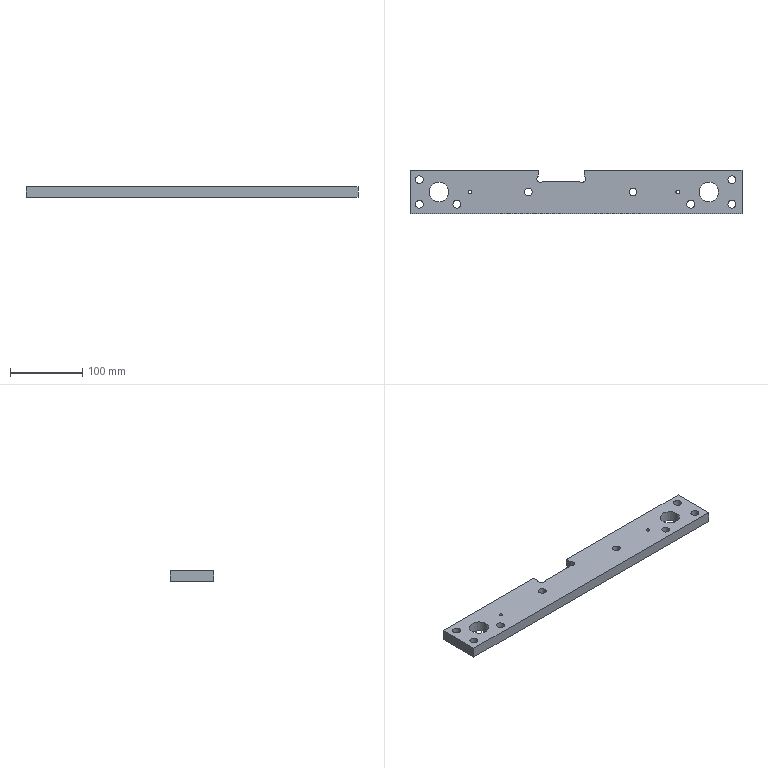Part | NX | features LIN_SOLID_COLOR 2 | 1 solid | 24 faces | box 460 x 60 x 15 mm | volume 369804 mm3 | cylinder 14 | plane 10 | commonest cylinder face diameters 11 x8 5.2 x2 10 x2 27 x2
STEP:
#1=CARTESIAN_POINT('',(813.,-110.,-46.5));
#2=VERTEX_POINT('',#1);
#3=CARTESIAN_POINT('',(594.5,-110.,-46.5));
#4=VERTEX_POINT('',#3);
#5=CARTESIAN_POINT('',(667.,-110.,-46.5));
#6=DIRECTION('',(-1.,0.,0.));
#7=VECTOR('',#6,1000.);
#8=LINE('',#5,#7);
#9=EDGE_CURVE('',#2,#4,#8,.T.);
#10=ORIENTED_EDGE('',*,*,#9,.T.);
#11=CARTESIAN_POINT('',(594.5,-110.,-31.5));
#12=VERTEX_POINT('',#11);
#13=CARTESIAN_POINT('',(594.5,-110.,-91.5));
#14=DIRECTION('',(0.,0.,1.));
#15=VECTOR('',#14,1000.);
#16=LINE('',#13,#15);
#17=EDGE_CURVE('',#12,#4,#16,.F.);
#18=ORIENTED_EDGE('',*,*,#17,.F.);
#19=CARTESIAN_POINT('',(813.,-110.,-31.5));
#20=VERTEX_POINT('',#19);
#21=CARTESIAN_POINT('',(667.,-110.,-31.5));
#22=DIRECTION('',(-1.,0.,0.));
#23=VECTOR('',#22,1000.);
#24=LINE('',#21,#23);
#25=EDGE_CURVE('',#12,#20,#24,.F.);
#26=ORIENTED_EDGE('',*,*,#25,.T.);
#27=CARTESIAN_POINT('',(813.,-110.,12.5));
#28=DIRECTION('',(0.,0.,1.));
#29=VECTOR('',#28,1000.);
#30=LINE('',#27,#29);
#31=EDGE_CURVE('',#2,#20,#30,.T.);
#32=ORIENTED_EDGE('',*,*,#31,.F.);
#33=EDGE_LOOP('',(#10,#18,#26,#32));
#34=FACE_BOUND('',#33,.T.);
#35=CARTESIAN_POINT('',(667.,-110.,-56.5));
#36=DIRECTION('',(0.,1.,0.));
#37=DIRECTION('',(0.,0.,1.));
#38=AXIS2_PLACEMENT_3D('',#35,#36,#37);
#39=PLANE('',#38);
#40=ADVANCED_FACE('',(#34),#39,.T.);
#41=CARTESIAN_POINT('',(353.,-110.,-31.5));
#42=VERTEX_POINT('',#41);
#43=CARTESIAN_POINT('',(530.5,-110.,-31.5));
#44=VERTEX_POINT('',#43);
#45=CARTESIAN_POINT('',(667.,-110.,-31.5));
#46=DIRECTION('',(-1.,0.,0.));
#47=VECTOR('',#46,1000.);
#48=LINE('',#45,#47);
#49=EDGE_CURVE('',#42,#44,#48,.F.);
#50=ORIENTED_EDGE('',*,*,#49,.T.);
#51=CARTESIAN_POINT('',(530.5,-110.,-46.5));
#52=VERTEX_POINT('',#51);
#53=CARTESIAN_POINT('',(530.5,-110.,-91.5));
#54=DIRECTION('',(0.,0.,1.));
#55=VECTOR('',#54,1000.);
#56=LINE('',#53,#55);
#57=EDGE_CURVE('',#52,#44,#56,.T.);
#58=ORIENTED_EDGE('',*,*,#57,.F.);
#59=CARTESIAN_POINT('',(353.,-110.,-46.5));
#60=VERTEX_POINT('',#59);
#61=CARTESIAN_POINT('',(667.,-110.,-46.5));
#62=DIRECTION('',(-1.,0.,0.));
#63=VECTOR('',#62,1000.);
#64=LINE('',#61,#63);
#65=EDGE_CURVE('',#52,#60,#64,.T.);
#66=ORIENTED_EDGE('',*,*,#65,.T.);
#67=CARTESIAN_POINT('',(353.,-110.,-56.5));
#68=DIRECTION('',(0.,0.,1.));
#69=VECTOR('',#68,1000.);
#70=LINE('',#67,#69);
#71=EDGE_CURVE('',#60,#42,#70,.T.);
#72=ORIENTED_EDGE('',*,*,#71,.T.);
#73=EDGE_LOOP('',(#50,#58,#66,#72));
#74=FACE_BOUND('',#73,.T.);
#75=CARTESIAN_POINT('',(667.,-110.,-56.5));
#76=DIRECTION('',(0.,1.,0.));
#77=DIRECTION('',(0.,0.,1.));
#78=AXIS2_PLACEMENT_3D('',#75,#76,#77);
#79=PLANE('',#78);
#80=ADVANCED_FACE('',(#74),#79,.T.);
#81=CARTESIAN_POINT('',(406.5,-140.,-31.5));
#82=VERTEX_POINT('',#81);
#83=CARTESIAN_POINT('',(393.,-140.,-31.5));
#84=DIRECTION('',(0.,0.,1.));
#85=DIRECTION('',(1.,0.,0.));
#86=AXIS2_PLACEMENT_3D('',#83,#84,#85);
#87=CIRCLE('',#86,13.5);
#88=EDGE_CURVE('',#82,#82,#87,.F.);
#89=ORIENTED_EDGE('',*,*,#88,.T.);
#90=EDGE_LOOP('',(#89));
#91=FACE_BOUND('',#90,.T.);
#92=CARTESIAN_POINT('',(753.5,-140.,-31.5));
#93=VERTEX_POINT('',#92);
#94=CARTESIAN_POINT('',(767.,-140.,-31.5));
#95=DIRECTION('',(0.,0.,-1.));
#96=DIRECTION('',(-1.,0.,0.));
#97=AXIS2_PLACEMENT_3D('',#94,#95,#96);
#98=CIRCLE('',#97,13.5);
#99=EDGE_CURVE('',#93,#93,#98,.F.);
#100=ORIENTED_EDGE('',*,*,#99,.F.);
#101=EDGE_LOOP('',(#100));
#102=FACE_BOUND('',#101,.T.);
#103=CARTESIAN_POINT('',(371.5,-123.,-31.5));
#104=VERTEX_POINT('',#103);
#105=CARTESIAN_POINT('',(366.,-123.,-31.5));
#106=DIRECTION('',(0.,0.,1.));
#107=DIRECTION('',(1.,0.,0.));
#108=AXIS2_PLACEMENT_3D('',#105,#106,#107);
#109=CIRCLE('',#108,5.5);
#110=EDGE_CURVE('',#104,#104,#109,.T.);
#111=ORIENTED_EDGE('',*,*,#110,.F.);
#112=EDGE_LOOP('',(#111));
#113=FACE_BOUND('',#112,.T.);
#114=CARTESIAN_POINT('',(522.5,-140.,-31.5));
#115=VERTEX_POINT('',#114);
#116=CARTESIAN_POINT('',(517.,-140.,-31.5));
#117=DIRECTION('',(0.,0.,1.));
#118=DIRECTION('',(1.,0.,0.));
#119=AXIS2_PLACEMENT_3D('',#116,#117,#118);
#120=CIRCLE('',#119,5.5);
#121=EDGE_CURVE('',#115,#115,#120,.T.);
#122=ORIENTED_EDGE('',*,*,#121,.F.);
#123=EDGE_LOOP('',(#122));
#124=FACE_BOUND('',#123,.T.);
#125=CARTESIAN_POINT('',(747.497,-157.,-31.5));
#126=VERTEX_POINT('',#125);
#127=CARTESIAN_POINT('',(741.997,-157.,-31.5));
#128=DIRECTION('',(0.,0.,1.));
#129=DIRECTION('',(1.,0.,0.));
#130=AXIS2_PLACEMENT_3D('',#127,#128,#129);
#131=CIRCLE('',#130,5.5);
#132=EDGE_CURVE('',#126,#126,#131,.T.);
#133=ORIENTED_EDGE('',*,*,#132,.F.);
#134=EDGE_LOOP('',(#133));
#135=FACE_BOUND('',#134,.T.);
#136=CARTESIAN_POINT('',(804.5,-157.,-31.5));
#137=VERTEX_POINT('',#136);
#138=CARTESIAN_POINT('',(799.,-157.,-31.5));
#139=DIRECTION('',(0.,0.,1.));
#140=DIRECTION('',(1.,0.,0.));
#141=AXIS2_PLACEMENT_3D('',#138,#139,#140);
#142=CIRCLE('',#141,5.5);
#143=EDGE_CURVE('',#137,#137,#142,.T.);
#144=ORIENTED_EDGE('',*,*,#143,.F.);
#145=EDGE_LOOP('',(#144));
#146=FACE_BOUND('',#145,.T.);
#147=CARTESIAN_POINT('',(804.5,-123.,-31.5));
#148=VERTEX_POINT('',#147);
#149=CARTESIAN_POINT('',(799.,-123.,-31.5));
#150=DIRECTION('',(0.,0.,1.));
#151=DIRECTION('',(1.,0.,0.));
#152=AXIS2_PLACEMENT_3D('',#149,#150,#151);
#153=CIRCLE('',#152,5.5);
#154=EDGE_CURVE('',#148,#148,#153,.T.);
#155=ORIENTED_EDGE('',*,*,#154,.F.);
#156=EDGE_LOOP('',(#155));
#157=FACE_BOUND('',#156,.T.);
#158=CARTESIAN_POINT('',(371.5,-157.,-31.5));
#159=VERTEX_POINT('',#158);
#160=CARTESIAN_POINT('',(366.,-157.,-31.5));
#161=DIRECTION('',(0.,0.,1.));
#162=DIRECTION('',(1.,0.,0.));
#163=AXIS2_PLACEMENT_3D('',#160,#161,#162);
#164=CIRCLE('',#163,5.5);
#165=EDGE_CURVE('',#159,#159,#164,.T.);
#166=ORIENTED_EDGE('',*,*,#165,.F.);
#167=EDGE_LOOP('',(#166));
#168=FACE_BOUND('',#167,.T.);
#169=CARTESIAN_POINT('',(423.503,-157.,-31.5));
#170=VERTEX_POINT('',#169);
#171=CARTESIAN_POINT('',(418.003,-157.,-31.5));
#172=DIRECTION('',(0.,0.,1.));
#173=DIRECTION('',(1.,0.,0.));
#174=AXIS2_PLACEMENT_3D('',#171,#172,#173);
#175=CIRCLE('',#174,5.5);
#176=EDGE_CURVE('',#170,#170,#175,.T.);
#177=ORIENTED_EDGE('',*,*,#176,.F.);
#178=EDGE_LOOP('',(#177));
#179=FACE_BOUND('',#178,.T.);
#180=CARTESIAN_POINT('',(726.6,-140.,-31.5));
#181=VERTEX_POINT('',#180);
#182=CARTESIAN_POINT('',(724.,-140.,-31.5));
#183=DIRECTION('',(0.,0.,1.));
#184=DIRECTION('',(1.,0.,0.));
#185=AXIS2_PLACEMENT_3D('',#182,#183,#184);
#186=CIRCLE('',#185,2.6);
#187=EDGE_CURVE('',#181,#181,#186,.T.);
#188=ORIENTED_EDGE('',*,*,#187,.F.);
#189=EDGE_LOOP('',(#188));
#190=FACE_BOUND('',#189,.T.);
#191=CARTESIAN_POINT('',(438.6,-140.,-31.5));
#192=VERTEX_POINT('',#191);
#193=CARTESIAN_POINT('',(436.,-140.,-31.5));
#194=DIRECTION('',(0.,0.,1.));
#195=DIRECTION('',(1.,0.,0.));
#196=AXIS2_PLACEMENT_3D('',#193,#194,#195);
#197=CIRCLE('',#196,2.6);
#198=EDGE_CURVE('',#192,#192,#197,.T.);
#199=ORIENTED_EDGE('',*,*,#198,.F.);
#200=EDGE_LOOP('',(#199));
#201=FACE_BOUND('',#200,.T.);
#202=CARTESIAN_POINT('',(667.5,-140.,-31.5));
#203=VERTEX_POINT('',#202);
#204=CARTESIAN_POINT('',(662.,-140.,-31.5));
#205=DIRECTION('',(0.,0.,1.));
#206=DIRECTION('',(1.,0.,0.));
#207=AXIS2_PLACEMENT_3D('',#204,#205,#206);
#208=CIRCLE('',#207,5.5);
#209=EDGE_CURVE('',#203,#203,#208,.T.);
#210=ORIENTED_EDGE('',*,*,#209,.F.);
#211=EDGE_LOOP('',(#210));
#212=FACE_BOUND('',#211,.T.);
#213=ORIENTED_EDGE('',*,*,#25,.F.);
#214=CARTESIAN_POINT('',(594.5,-117.961,-31.5));
#215=VERTEX_POINT('',#214);
#216=CARTESIAN_POINT('',(594.5,-140.,-31.5));
#217=DIRECTION('',(0.,-1.,0.));
#218=VECTOR('',#217,1000.);
#219=LINE('',#216,#218);
#220=EDGE_CURVE('',#215,#12,#219,.F.);
#221=ORIENTED_EDGE('',*,*,#220,.F.);
#222=CARTESIAN_POINT('',(587.461,-125.,-31.5));
#223=VERTEX_POINT('',#222);
#224=CARTESIAN_POINT('',(591.318,-121.818,-31.5));
#225=DIRECTION('',(0.,0.,1.));
#226=DIRECTION('',(1.,0.,0.));
#227=AXIS2_PLACEMENT_3D('',#224,#225,#226);
#228=CIRCLE('',#227,5.);
#229=EDGE_CURVE('',#223,#215,#228,.T.);
#230=ORIENTED_EDGE('',*,*,#229,.F.);
#231=CARTESIAN_POINT('',(537.539,-125.,-31.5));
#232=VERTEX_POINT('',#231);
#233=CARTESIAN_POINT('',(667.,-125.,-31.5));
#234=DIRECTION('',(-1.,0.,0.));
#235=VECTOR('',#234,1000.);
#236=LINE('',#233,#235);
#237=EDGE_CURVE('',#232,#223,#236,.F.);
#238=ORIENTED_EDGE('',*,*,#237,.F.);
#239=CARTESIAN_POINT('',(530.5,-117.961,-31.5));
#240=VERTEX_POINT('',#239);
#241=CARTESIAN_POINT('',(533.682,-121.818,-31.5));
#242=DIRECTION('',(0.,0.,1.));
#243=DIRECTION('',(1.,0.,0.));
#244=AXIS2_PLACEMENT_3D('',#241,#242,#243);
#245=CIRCLE('',#244,5.);
#246=EDGE_CURVE('',#232,#240,#245,.F.);
#247=ORIENTED_EDGE('',*,*,#246,.T.);
#248=CARTESIAN_POINT('',(530.5,-140.,-31.5));
#249=DIRECTION('',(0.,1.,0.));
#250=VECTOR('',#249,1000.);
#251=LINE('',#248,#250);
#252=EDGE_CURVE('',#240,#44,#251,.T.);
#253=ORIENTED_EDGE('',*,*,#252,.T.);
#254=ORIENTED_EDGE('',*,*,#49,.F.);
#255=CARTESIAN_POINT('',(353.,-170.,-31.5));
#256=VERTEX_POINT('',#255);
#257=CARTESIAN_POINT('',(353.,-30.,-31.5));
#258=DIRECTION('',(0.,1.,0.));
#259=VECTOR('',#258,1000.);
#260=LINE('',#257,#259);
#261=EDGE_CURVE('',#256,#42,#260,.T.);
#262=ORIENTED_EDGE('',*,*,#261,.F.);
#263=CARTESIAN_POINT('',(813.,-170.,-31.5));
#264=VERTEX_POINT('',#263);
#265=CARTESIAN_POINT('',(667.,-170.,-31.5));
#266=DIRECTION('',(1.,0.,0.));
#267=VECTOR('',#266,1000.);
#268=LINE('',#265,#267);
#269=EDGE_CURVE('',#264,#256,#268,.F.);
#270=ORIENTED_EDGE('',*,*,#269,.F.);
#271=CARTESIAN_POINT('',(813.,-140.,-31.5));
#272=DIRECTION('',(0.,1.,0.));
#273=VECTOR('',#272,1000.);
#274=LINE('',#271,#273);
#275=EDGE_CURVE('',#264,#20,#274,.T.);
#276=ORIENTED_EDGE('',*,*,#275,.T.);
#277=EDGE_LOOP('',(#213,#221,#230,#238,#247,#253,#254,#262,#270,#276));
#278=FACE_BOUND('',#277,.T.);
#279=CARTESIAN_POINT('',(667.,-140.,-31.5));
#280=DIRECTION('',(0.,0.,1.));
#281=DIRECTION('',(-1.,0.,0.));
#282=AXIS2_PLACEMENT_3D('',#279,#280,#281);
#283=PLANE('',#282);
#284=ADVANCED_FACE('',(#91,#102,#113,#124,#135,#146,#157,#168,#179,#190,#201,#212,#278),#283,.T.);
#285=CARTESIAN_POINT('',(433.4,-140.,-46.5));
#286=VERTEX_POINT('',#285);
#287=CARTESIAN_POINT('',(436.,-140.,-46.5));
#288=DIRECTION('',(0.,0.,-1.));
#289=DIRECTION('',(-1.,0.,0.));
#290=AXIS2_PLACEMENT_3D('',#287,#288,#289);
#291=CIRCLE('',#290,2.6);
#292=EDGE_CURVE('',#286,#286,#291,.F.);
#293=ORIENTED_EDGE('',*,*,#292,.T.);
#294=EDGE_LOOP('',(#293));
#295=FACE_BOUND('',#294,.T.);
#296=CARTESIAN_POINT('',(379.5,-140.,-46.5));
#297=VERTEX_POINT('',#296);
#298=CARTESIAN_POINT('',(393.,-140.,-46.5));
#299=DIRECTION('',(0.,0.,-1.));
#300=DIRECTION('',(-1.,0.,0.));
#301=AXIS2_PLACEMENT_3D('',#298,#299,#300);
#302=CIRCLE('',#301,13.5);
#303=EDGE_CURVE('',#297,#297,#302,.F.);
#304=ORIENTED_EDGE('',*,*,#303,.T.);
#305=EDGE_LOOP('',(#304));
#306=FACE_BOUND('',#305,.T.);
#307=CARTESIAN_POINT('',(753.5,-140.,-46.5));
#308=VERTEX_POINT('',#307);
#309=CARTESIAN_POINT('',(767.,-140.,-46.5));
#310=DIRECTION('',(0.,0.,-1.));
#311=DIRECTION('',(-1.,0.,0.));
#312=AXIS2_PLACEMENT_3D('',#309,#310,#311);
#313=CIRCLE('',#312,13.5);
#314=EDGE_CURVE('',#308,#308,#313,.T.);
#315=ORIENTED_EDGE('',*,*,#314,.F.);
#316=EDGE_LOOP('',(#315));
#317=FACE_BOUND('',#316,.T.);
#318=CARTESIAN_POINT('',(360.5,-123.,-46.5));
#319=VERTEX_POINT('',#318);
#320=CARTESIAN_POINT('',(366.,-123.,-46.5));
#321=DIRECTION('',(0.,0.,-1.));
#322=DIRECTION('',(-1.,0.,0.));
#323=AXIS2_PLACEMENT_3D('',#320,#321,#322);
#324=CIRCLE('',#323,5.5);
#325=EDGE_CURVE('',#319,#319,#324,.T.);
#326=ORIENTED_EDGE('',*,*,#325,.F.);
#327=EDGE_LOOP('',(#326));
#328=FACE_BOUND('',#327,.T.);
#329=CARTESIAN_POINT('',(511.5,-140.,-46.5));
#330=VERTEX_POINT('',#329);
#331=CARTESIAN_POINT('',(517.,-140.,-46.5));
#332=DIRECTION('',(0.,0.,-1.));
#333=DIRECTION('',(-1.,0.,0.));
#334=AXIS2_PLACEMENT_3D('',#331,#332,#333);
#335=CIRCLE('',#334,5.5);
#336=EDGE_CURVE('',#330,#330,#335,.T.);
#337=ORIENTED_EDGE('',*,*,#336,.F.);
#338=EDGE_LOOP('',(#337));
#339=FACE_BOUND('',#338,.T.);
#340=CARTESIAN_POINT('',(736.497,-157.,-46.5));
#341=VERTEX_POINT('',#340);
#342=CARTESIAN_POINT('',(741.997,-157.,-46.5));
#343=DIRECTION('',(0.,0.,-1.));
#344=DIRECTION('',(-1.,0.,0.));
#345=AXIS2_PLACEMENT_3D('',#342,#343,#344);
#346=CIRCLE('',#345,5.5);
#347=EDGE_CURVE('',#341,#341,#346,.T.);
#348=ORIENTED_EDGE('',*,*,#347,.F.);
#349=EDGE_LOOP('',(#348));
#350=FACE_BOUND('',#349,.T.);
#351=CARTESIAN_POINT('',(793.5,-157.,-46.5));
#352=VERTEX_POINT('',#351);
#353=CARTESIAN_POINT('',(799.,-157.,-46.5));
#354=DIRECTION('',(0.,0.,-1.));
#355=DIRECTION('',(-1.,0.,0.));
#356=AXIS2_PLACEMENT_3D('',#353,#354,#355);
#357=CIRCLE('',#356,5.5);
#358=EDGE_CURVE('',#352,#352,#357,.T.);
#359=ORIENTED_EDGE('',*,*,#358,.F.);
#360=EDGE_LOOP('',(#359));
#361=FACE_BOUND('',#360,.T.);
#362=CARTESIAN_POINT('',(793.5,-123.,-46.5));
#363=VERTEX_POINT('',#362);
#364=CARTESIAN_POINT('',(799.,-123.,-46.5));
#365=DIRECTION('',(0.,0.,-1.));
#366=DIRECTION('',(-1.,0.,0.));
#367=AXIS2_PLACEMENT_3D('',#364,#365,#366);
#368=CIRCLE('',#367,5.5);
#369=EDGE_CURVE('',#363,#363,#368,.T.);
#370=ORIENTED_EDGE('',*,*,#369,.F.);
#371=EDGE_LOOP('',(#370));
#372=FACE_BOUND('',#371,.T.);
#373=CARTESIAN_POINT('',(360.5,-157.,-46.5));
#374=VERTEX_POINT('',#373);
#375=CARTESIAN_POINT('',(366.,-157.,-46.5));
#376=DIRECTION('',(0.,0.,-1.));
#377=DIRECTION('',(-1.,0.,0.));
#378=AXIS2_PLACEMENT_3D('',#375,#376,#377);
#379=CIRCLE('',#378,5.5);
#380=EDGE_CURVE('',#374,#374,#379,.T.);
#381=ORIENTED_EDGE('',*,*,#380,.F.);
#382=EDGE_LOOP('',(#381));
#383=FACE_BOUND('',#382,.T.);
#384=CARTESIAN_POINT('',(412.503,-157.,-46.5));
#385=VERTEX_POINT('',#384);
#386=CARTESIAN_POINT('',(418.003,-157.,-46.5));
#387=DIRECTION('',(0.,0.,-1.));
#388=DIRECTION('',(-1.,0.,0.));
#389=AXIS2_PLACEMENT_3D('',#386,#387,#388);
#390=CIRCLE('',#389,5.5);
#391=EDGE_CURVE('',#385,#385,#390,.T.);
#392=ORIENTED_EDGE('',*,*,#391,.F.);
#393=EDGE_LOOP('',(#392));
#394=FACE_BOUND('',#393,.T.);
#395=CARTESIAN_POINT('',(721.4,-140.,-46.5));
#396=VERTEX_POINT('',#395);
#397=CARTESIAN_POINT('',(724.,-140.,-46.5));
#398=DIRECTION('',(0.,0.,-1.));
#399=DIRECTION('',(-1.,0.,0.));
#400=AXIS2_PLACEMENT_3D('',#397,#398,#399);
#401=CIRCLE('',#400,2.6);
#402=EDGE_CURVE('',#396,#396,#401,.F.);
#403=ORIENTED_EDGE('',*,*,#402,.T.);
#404=EDGE_LOOP('',(#403));
#405=FACE_BOUND('',#404,.T.);
#406=CARTESIAN_POINT('',(656.5,-140.,-46.5));
#407=VERTEX_POINT('',#406);
#408=CARTESIAN_POINT('',(662.,-140.,-46.5));
#409=DIRECTION('',(0.,0.,-1.));
#410=DIRECTION('',(-1.,0.,0.));
#411=AXIS2_PLACEMENT_3D('',#408,#409,#410);
#412=CIRCLE('',#411,5.5);
#413=EDGE_CURVE('',#407,#407,#412,.T.);
#414=ORIENTED_EDGE('',*,*,#413,.F.);
#415=EDGE_LOOP('',(#414));
#416=FACE_BOUND('',#415,.T.);
#417=CARTESIAN_POINT('',(587.461,-125.,-46.5));
#418=VERTEX_POINT('',#417);
#419=CARTESIAN_POINT('',(594.5,-117.961,-46.5));
#420=VERTEX_POINT('',#419);
#421=CARTESIAN_POINT('',(591.318,-121.818,-46.5));
#422=DIRECTION('',(0.,0.,-1.));
#423=DIRECTION('',(-1.,0.,0.));
#424=AXIS2_PLACEMENT_3D('',#421,#422,#423);
#425=CIRCLE('',#424,5.);
#426=EDGE_CURVE('',#418,#420,#425,.F.);
#427=ORIENTED_EDGE('',*,*,#426,.T.);
#428=CARTESIAN_POINT('',(594.5,-140.,-46.5));
#429=DIRECTION('',(0.,1.,0.));
#430=VECTOR('',#429,1000.);
#431=LINE('',#428,#430);
#432=EDGE_CURVE('',#4,#420,#431,.F.);
#433=ORIENTED_EDGE('',*,*,#432,.F.);
#434=ORIENTED_EDGE('',*,*,#9,.F.);
#435=CARTESIAN_POINT('',(813.,-170.,-46.5));
#436=VERTEX_POINT('',#435);
#437=CARTESIAN_POINT('',(813.,-140.,-46.5));
#438=DIRECTION('',(0.,-1.,0.));
#439=VECTOR('',#438,1000.);
#440=LINE('',#437,#439);
#441=EDGE_CURVE('',#2,#436,#440,.T.);
#442=ORIENTED_EDGE('',*,*,#441,.T.);
#443=CARTESIAN_POINT('',(353.,-170.,-46.5));
#444=VERTEX_POINT('',#443);
#445=CARTESIAN_POINT('',(667.,-170.,-46.5));
#446=DIRECTION('',(1.,0.,0.));
#447=VECTOR('',#446,1000.);
#448=LINE('',#445,#447);
#449=EDGE_CURVE('',#444,#436,#448,.T.);
#450=ORIENTED_EDGE('',*,*,#449,.F.);
#451=CARTESIAN_POINT('',(353.,-30.,-46.5));
#452=DIRECTION('',(0.,-1.,0.));
#453=VECTOR('',#452,1000.);
#454=LINE('',#451,#453);
#455=EDGE_CURVE('',#60,#444,#454,.T.);
#456=ORIENTED_EDGE('',*,*,#455,.F.);
#457=ORIENTED_EDGE('',*,*,#65,.F.);
#458=CARTESIAN_POINT('',(530.5,-117.961,-46.5));
#459=VERTEX_POINT('',#458);
#460=CARTESIAN_POINT('',(530.5,-140.,-46.5));
#461=DIRECTION('',(0.,-1.,0.));
#462=VECTOR('',#461,1000.);
#463=LINE('',#460,#462);
#464=EDGE_CURVE('',#459,#52,#463,.F.);
#465=ORIENTED_EDGE('',*,*,#464,.F.);
#466=CARTESIAN_POINT('',(537.539,-125.,-46.5));
#467=VERTEX_POINT('',#466);
#468=CARTESIAN_POINT('',(533.682,-121.818,-46.5));
#469=DIRECTION('',(0.,0.,-1.));
#470=DIRECTION('',(-1.,0.,0.));
#471=AXIS2_PLACEMENT_3D('',#468,#469,#470);
#472=CIRCLE('',#471,5.);
#473=EDGE_CURVE('',#459,#467,#472,.F.);
#474=ORIENTED_EDGE('',*,*,#473,.T.);
#475=CARTESIAN_POINT('',(667.,-125.,-46.5));
#476=DIRECTION('',(1.,0.,0.));
#477=VECTOR('',#476,1000.);
#478=LINE('',#475,#477);
#479=EDGE_CURVE('',#467,#418,#478,.T.);
#480=ORIENTED_EDGE('',*,*,#479,.T.);
#481=EDGE_LOOP('',(#427,#433,#434,#442,#450,#456,#457,#465,#474,#480));
#482=FACE_BOUND('',#481,.T.);
#483=CARTESIAN_POINT('',(667.,-140.,-46.5));
#484=DIRECTION('',(0.,0.,-1.));
#485=DIRECTION('',(1.,0.,0.));
#486=AXIS2_PLACEMENT_3D('',#483,#484,#485);
#487=PLANE('',#486);
#488=ADVANCED_FACE('',(#295,#306,#317,#328,#339,#350,#361,#372,#383,#394,#405,#416,#482),#487,.T.);
#489=ORIENTED_EDGE('',*,*,#209,.T.);
#490=EDGE_LOOP('',(#489));
#491=FACE_BOUND('',#490,.T.);
#492=ORIENTED_EDGE('',*,*,#413,.T.);
#493=EDGE_LOOP('',(#492));
#494=FACE_BOUND('',#493,.T.);
#495=CARTESIAN_POINT('',(662.,-140.,-31.4));
#496=DIRECTION('',(0.,0.,-1.));
#497=DIRECTION('',(1.,0.,0.));
#498=AXIS2_PLACEMENT_3D('',#495,#496,#497);
#499=CYLINDRICAL_SURFACE('',#498,5.5);
#500=ADVANCED_FACE('',(#491,#494),#499,.F.);
#501=ORIENTED_EDGE('',*,*,#88,.F.);
#502=EDGE_LOOP('',(#501));
#503=FACE_BOUND('',#502,.T.);
#504=ORIENTED_EDGE('',*,*,#303,.F.);
#505=EDGE_LOOP('',(#504));
#506=FACE_BOUND('',#505,.T.);
#507=CARTESIAN_POINT('',(393.,-140.,-1.));
#508=DIRECTION('',(0.,0.,-1.));
#509=DIRECTION('',(-1.,0.,0.));
#510=AXIS2_PLACEMENT_3D('',#507,#508,#509);
#511=CYLINDRICAL_SURFACE('',#510,13.5);
#512=ADVANCED_FACE('',(#503,#506),#511,.F.);
#513=ORIENTED_EDGE('',*,*,#99,.T.);
#514=EDGE_LOOP('',(#513));
#515=FACE_BOUND('',#514,.T.);
#516=ORIENTED_EDGE('',*,*,#314,.T.);
#517=EDGE_LOOP('',(#516));
#518=FACE_BOUND('',#517,.T.);
#519=CARTESIAN_POINT('',(767.,-140.,-1.));
#520=DIRECTION('',(0.,0.,-1.));
#521=DIRECTION('',(1.,0.,0.));
#522=AXIS2_PLACEMENT_3D('',#519,#520,#521);
#523=CYLINDRICAL_SURFACE('',#522,13.5);
#524=ADVANCED_FACE('',(#515,#518),#523,.F.);
#525=CARTESIAN_POINT('',(353.,-170.,25.));
#526=DIRECTION('',(0.,0.,1.));
#527=VECTOR('',#526,1000.);
#528=LINE('',#525,#527);
#529=EDGE_CURVE('',#444,#256,#528,.T.);
#530=ORIENTED_EDGE('',*,*,#529,.T.);
#531=ORIENTED_EDGE('',*,*,#261,.T.);
#532=ORIENTED_EDGE('',*,*,#71,.F.);
#533=ORIENTED_EDGE('',*,*,#455,.T.);
#534=EDGE_LOOP('',(#530,#531,#532,#533));
#535=FACE_BOUND('',#534,.T.);
#536=CARTESIAN_POINT('',(353.,-30.,25.));
#537=DIRECTION('',(-1.,0.,0.));
#538=DIRECTION('',(0.,0.,1.));
#539=AXIS2_PLACEMENT_3D('',#536,#537,#538);
#540=PLANE('',#539);
#541=ADVANCED_FACE('',(#535),#540,.T.);
#542=CARTESIAN_POINT('',(813.,-170.,-56.5));
#543=DIRECTION('',(0.,0.,1.));
#544=VECTOR('',#543,1000.);
#545=LINE('',#542,#544);
#546=EDGE_CURVE('',#436,#264,#545,.T.);
#547=ORIENTED_EDGE('',*,*,#546,.F.);
#548=ORIENTED_EDGE('',*,*,#441,.F.);
#549=ORIENTED_EDGE('',*,*,#31,.T.);
#550=ORIENTED_EDGE('',*,*,#275,.F.);
#551=EDGE_LOOP('',(#547,#548,#549,#550));
#552=FACE_BOUND('',#551,.T.);
#553=CARTESIAN_POINT('',(813.,-30.,12.5));
#554=DIRECTION('',(1.,0.,0.));
#555=DIRECTION('',(0.,0.,-1.));
#556=AXIS2_PLACEMENT_3D('',#553,#554,#555);
#557=PLANE('',#556);
#558=ADVANCED_FACE('',(#552),#557,.T.);
#559=ORIENTED_EDGE('',*,*,#269,.T.);
#560=ORIENTED_EDGE('',*,*,#529,.F.);
#561=ORIENTED_EDGE('',*,*,#449,.T.);
#562=ORIENTED_EDGE('',*,*,#546,.T.);
#563=EDGE_LOOP('',(#559,#560,#561,#562));
#564=FACE_BOUND('',#563,.T.);
#565=CARTESIAN_POINT('',(667.,-170.,-56.5));
#566=DIRECTION('',(0.,-1.,0.));
#567=DIRECTION('',(0.,0.,-1.));
#568=AXIS2_PLACEMENT_3D('',#565,#566,#567);
#569=PLANE('',#568);
#570=ADVANCED_FACE('',(#564),#569,.T.);
#571=ORIENTED_EDGE('',*,*,#110,.T.);
#572=EDGE_LOOP('',(#571));
#573=FACE_BOUND('',#572,.T.);
#574=ORIENTED_EDGE('',*,*,#325,.T.);
#575=EDGE_LOOP('',(#574));
#576=FACE_BOUND('',#575,.T.);
#577=CARTESIAN_POINT('',(366.,-123.,-31.4));
#578=DIRECTION('',(0.,0.,-1.));
#579=DIRECTION('',(1.,0.,0.));
#580=AXIS2_PLACEMENT_3D('',#577,#578,#579);
#581=CYLINDRICAL_SURFACE('',#580,5.5);
#582=ADVANCED_FACE('',(#573,#576),#581,.F.);
#583=ORIENTED_EDGE('',*,*,#121,.T.);
#584=EDGE_LOOP('',(#583));
#585=FACE_BOUND('',#584,.T.);
#586=ORIENTED_EDGE('',*,*,#336,.T.);
#587=EDGE_LOOP('',(#586));
#588=FACE_BOUND('',#587,.T.);
#589=CARTESIAN_POINT('',(517.,-140.,-31.4));
#590=DIRECTION('',(0.,0.,-1.));
#591=DIRECTION('',(1.,0.,0.));
#592=AXIS2_PLACEMENT_3D('',#589,#590,#591);
#593=CYLINDRICAL_SURFACE('',#592,5.5);
#594=ADVANCED_FACE('',(#585,#588),#593,.F.);
#595=ORIENTED_EDGE('',*,*,#132,.T.);
#596=EDGE_LOOP('',(#595));
#597=FACE_BOUND('',#596,.T.);
#598=ORIENTED_EDGE('',*,*,#347,.T.);
#599=EDGE_LOOP('',(#598));
#600=FACE_BOUND('',#599,.T.);
#601=CARTESIAN_POINT('',(741.997,-157.,-31.4));
#602=DIRECTION('',(0.,0.,-1.));
#603=DIRECTION('',(1.,0.,0.));
#604=AXIS2_PLACEMENT_3D('',#601,#602,#603);
#605=CYLINDRICAL_SURFACE('',#604,5.5);
#606=ADVANCED_FACE('',(#597,#600),#605,.F.);
#607=ORIENTED_EDGE('',*,*,#143,.T.);
#608=EDGE_LOOP('',(#607));
#609=FACE_BOUND('',#608,.T.);
#610=ORIENTED_EDGE('',*,*,#358,.T.);
#611=EDGE_LOOP('',(#610));
#612=FACE_BOUND('',#611,.T.);
#613=CARTESIAN_POINT('',(799.,-157.,-31.4));
#614=DIRECTION('',(0.,0.,-1.));
#615=DIRECTION('',(1.,0.,0.));
#616=AXIS2_PLACEMENT_3D('',#613,#614,#615);
#617=CYLINDRICAL_SURFACE('',#616,5.5);
#618=ADVANCED_FACE('',(#609,#612),#617,.F.);
#619=ORIENTED_EDGE('',*,*,#154,.T.);
#620=EDGE_LOOP('',(#619));
#621=FACE_BOUND('',#620,.T.);
#622=ORIENTED_EDGE('',*,*,#369,.T.);
#623=EDGE_LOOP('',(#622));
#624=FACE_BOUND('',#623,.T.);
#625=CARTESIAN_POINT('',(799.,-123.,-31.4));
#626=DIRECTION('',(0.,0.,-1.));
#627=DIRECTION('',(1.,0.,0.));
#628=AXIS2_PLACEMENT_3D('',#625,#626,#627);
#629=CYLINDRICAL_SURFACE('',#628,5.5);
#630=ADVANCED_FACE('',(#621,#624),#629,.F.);
#631=ORIENTED_EDGE('',*,*,#165,.T.);
#632=EDGE_LOOP('',(#631));
#633=FACE_BOUND('',#632,.T.);
#634=ORIENTED_EDGE('',*,*,#380,.T.);
#635=EDGE_LOOP('',(#634));
#636=FACE_BOUND('',#635,.T.);
#637=CARTESIAN_POINT('',(366.,-157.,-31.4));
#638=DIRECTION('',(0.,0.,-1.));
#639=DIRECTION('',(1.,0.,0.));
#640=AXIS2_PLACEMENT_3D('',#637,#638,#639);
#641=CYLINDRICAL_SURFACE('',#640,5.5);
#642=ADVANCED_FACE('',(#633,#636),#641,.F.);
#643=ORIENTED_EDGE('',*,*,#176,.T.);
#644=EDGE_LOOP('',(#643));
#645=FACE_BOUND('',#644,.T.);
#646=ORIENTED_EDGE('',*,*,#391,.T.);
#647=EDGE_LOOP('',(#646));
#648=FACE_BOUND('',#647,.T.);
#649=CARTESIAN_POINT('',(418.003,-157.,-31.4));
#650=DIRECTION('',(0.,0.,-1.));
#651=DIRECTION('',(1.,0.,0.));
#652=AXIS2_PLACEMENT_3D('',#649,#650,#651);
#653=CYLINDRICAL_SURFACE('',#652,5.5);
#654=ADVANCED_FACE('',(#645,#648),#653,.F.);
#655=ORIENTED_EDGE('',*,*,#402,.F.);
#656=EDGE_LOOP('',(#655));
#657=FACE_BOUND('',#656,.T.);
#658=ORIENTED_EDGE('',*,*,#187,.T.);
#659=EDGE_LOOP('',(#658));
#660=FACE_BOUND('',#659,.T.);
#661=CARTESIAN_POINT('',(724.,-140.,-31.4));
#662=DIRECTION('',(0.,0.,-1.));
#663=DIRECTION('',(1.,0.,0.));
#664=AXIS2_PLACEMENT_3D('',#661,#662,#663);
#665=CYLINDRICAL_SURFACE('',#664,2.6);
#666=ADVANCED_FACE('',(#657,#660),#665,.F.);
#667=ORIENTED_EDGE('',*,*,#292,.F.);
#668=EDGE_LOOP('',(#667));
#669=FACE_BOUND('',#668,.T.);
#670=ORIENTED_EDGE('',*,*,#198,.T.);
#671=EDGE_LOOP('',(#670));
#672=FACE_BOUND('',#671,.T.);
#673=CARTESIAN_POINT('',(436.,-140.,-31.4));
#674=DIRECTION('',(0.,0.,-1.));
#675=DIRECTION('',(1.,0.,0.));
#676=AXIS2_PLACEMENT_3D('',#673,#674,#675);
#677=CYLINDRICAL_SURFACE('',#676,2.6);
#678=ADVANCED_FACE('',(#669,#672),#677,.F.);
#679=ORIENTED_EDGE('',*,*,#246,.F.);
#680=CARTESIAN_POINT('',(537.539,-125.,-121.5));
#681=DIRECTION('',(0.,0.,1.));
#682=VECTOR('',#681,1000.);
#683=LINE('',#680,#682);
#684=EDGE_CURVE('',#467,#232,#683,.T.);
#685=ORIENTED_EDGE('',*,*,#684,.F.);
#686=ORIENTED_EDGE('',*,*,#473,.F.);
#687=CARTESIAN_POINT('',(530.5,-117.961,-91.5));
#688=DIRECTION('',(0.,0.,1.));
#689=VECTOR('',#688,1000.);
#690=LINE('',#687,#689);
#691=EDGE_CURVE('',#240,#459,#690,.F.);
#692=ORIENTED_EDGE('',*,*,#691,.F.);
#693=EDGE_LOOP('',(#679,#685,#686,#692));
#694=FACE_BOUND('',#693,.T.);
#695=CARTESIAN_POINT('',(533.682,-121.818,-121.5));
#696=DIRECTION('',(0.,0.,1.));
#697=DIRECTION('',(1.,0.,0.));
#698=AXIS2_PLACEMENT_3D('',#695,#696,#697);
#699=CYLINDRICAL_SURFACE('',#698,5.);
#700=ADVANCED_FACE('',(#694),#699,.F.);
#701=ORIENTED_EDGE('',*,*,#220,.T.);
#702=ORIENTED_EDGE('',*,*,#17,.T.);
#703=ORIENTED_EDGE('',*,*,#432,.T.);
#704=CARTESIAN_POINT('',(594.5,-117.961,-91.5));
#705=DIRECTION('',(0.,0.,1.));
#706=VECTOR('',#705,1000.);
#707=LINE('',#704,#706);
#708=EDGE_CURVE('',#420,#215,#707,.T.);
#709=ORIENTED_EDGE('',*,*,#708,.T.);
#710=EDGE_LOOP('',(#701,#702,#703,#709));
#711=FACE_BOUND('',#710,.T.);
#712=CARTESIAN_POINT('',(594.5,-110.,-91.5));
#713=DIRECTION('',(-1.,0.,0.));
#714=DIRECTION('',(0.,0.,1.));
#715=AXIS2_PLACEMENT_3D('',#712,#713,#714);
#716=PLANE('',#715);
#717=ADVANCED_FACE('',(#711),#716,.T.);
#718=ORIENTED_EDGE('',*,*,#229,.T.);
#719=ORIENTED_EDGE('',*,*,#708,.F.);
#720=ORIENTED_EDGE('',*,*,#426,.F.);
#721=CARTESIAN_POINT('',(587.461,-125.,-91.5));
#722=DIRECTION('',(0.,0.,1.));
#723=VECTOR('',#722,1000.);
#724=LINE('',#721,#723);
#725=EDGE_CURVE('',#418,#223,#724,.T.);
#726=ORIENTED_EDGE('',*,*,#725,.T.);
#727=EDGE_LOOP('',(#718,#719,#720,#726));
#728=FACE_BOUND('',#727,.T.);
#729=CARTESIAN_POINT('',(591.318,-121.818,-91.5));
#730=DIRECTION('',(0.,0.,1.));
#731=DIRECTION('',(1.,0.,0.));
#732=AXIS2_PLACEMENT_3D('',#729,#730,#731);
#733=CYLINDRICAL_SURFACE('',#732,5.);
#734=ADVANCED_FACE('',(#728),#733,.F.);
#735=ORIENTED_EDGE('',*,*,#237,.T.);
#736=ORIENTED_EDGE('',*,*,#725,.F.);
#737=ORIENTED_EDGE('',*,*,#479,.F.);
#738=ORIENTED_EDGE('',*,*,#684,.T.);
#739=EDGE_LOOP('',(#735,#736,#737,#738));
#740=FACE_BOUND('',#739,.T.);
#741=CARTESIAN_POINT('',(587.461,-125.,-91.5));
#742=DIRECTION('',(0.,1.,0.));
#743=DIRECTION('',(0.,0.,1.));
#744=AXIS2_PLACEMENT_3D('',#741,#742,#743);
#745=PLANE('',#744);
#746=ADVANCED_FACE('',(#740),#745,.T.);
#747=ORIENTED_EDGE('',*,*,#252,.F.);
#748=ORIENTED_EDGE('',*,*,#691,.T.);
#749=ORIENTED_EDGE('',*,*,#464,.T.);
#750=ORIENTED_EDGE('',*,*,#57,.T.);
#751=EDGE_LOOP('',(#747,#748,#749,#750));
#752=FACE_BOUND('',#751,.T.);
#753=CARTESIAN_POINT('',(530.5,-114.961,-91.5));
#754=DIRECTION('',(1.,0.,0.));
#755=DIRECTION('',(0.,0.,-1.));
#756=AXIS2_PLACEMENT_3D('',#753,#754,#755);
#757=PLANE('',#756);
#758=ADVANCED_FACE('',(#752),#757,.T.);
#759=CLOSED_SHELL('',(#40,#80,#284,#488,#500,#512,#524,#541,#558,#570,#582,#594,#606,#618,#630,#642,#654,#666,#678,#700,#717,#734,#746,#758));
#760=MANIFOLD_SOLID_BREP('',#759);
#761=(LENGTH_UNIT()NAMED_UNIT(*)SI_UNIT(.MILLI.,.METRE.));
#762=UNCERTAINTY_MEASURE_WITH_UNIT(LENGTH_MEASURE(0.00001),#761,'','');
#763=(NAMED_UNIT(*)PLANE_ANGLE_UNIT()SI_UNIT($,.RADIAN.));
#764=(NAMED_UNIT(*)SI_UNIT($,.STERADIAN.)SOLID_ANGLE_UNIT());
#765=(GEOMETRIC_REPRESENTATION_CONTEXT(3)GLOBAL_UNCERTAINTY_ASSIGNED_CONTEXT((#762))GLOBAL_UNIT_ASSIGNED_CONTEXT((#761,#763,#764))REPRESENTATION_CONTEXT('',''));
#766=ADVANCED_BREP_SHAPE_REPRESENTATION('',(#760),#765);